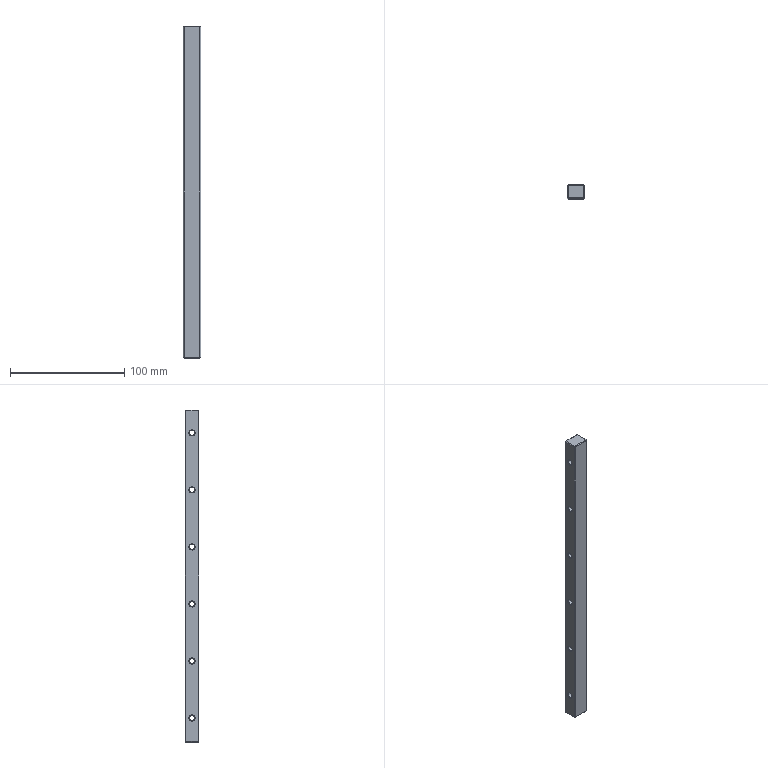Part | STEP file | Clip jig-column 1 | 1 solid | 87 faces | box 15 x 12 x 291 mm | volume 49759 mm3 | plane 33 | cylinder 28 | cone 26 | commonest cylinder face diameters 4.5 x12 8 x12 3.3 x4